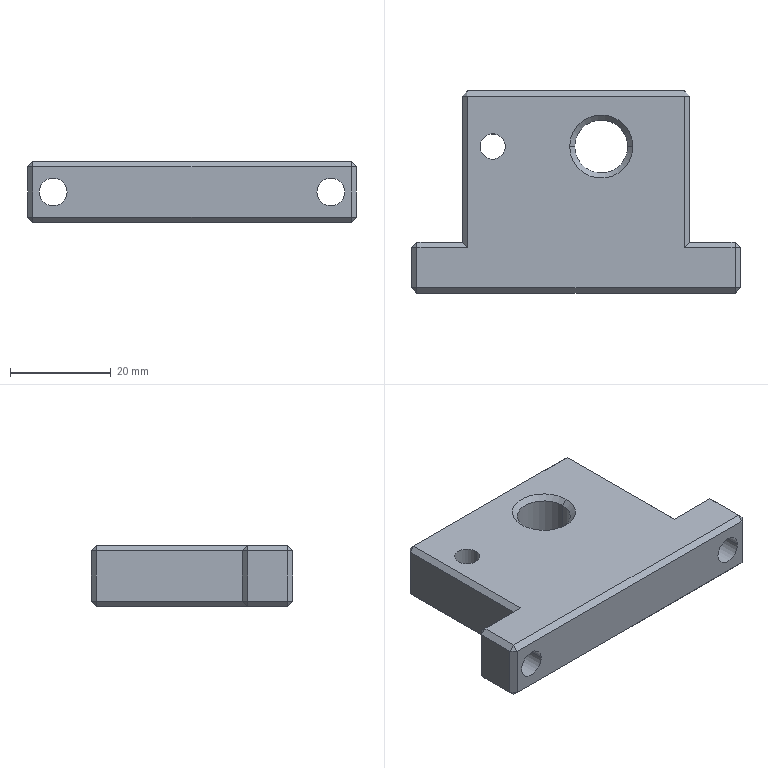Part | STEP file | 1 solid | 56 faces | box 65 x 40 x 12 mm | volume 21976 mm3 | plane 44 | cylinder 8 | cone 4 | commonest cylinder face diameters 5.5 x4 5 x2 10.5 x2